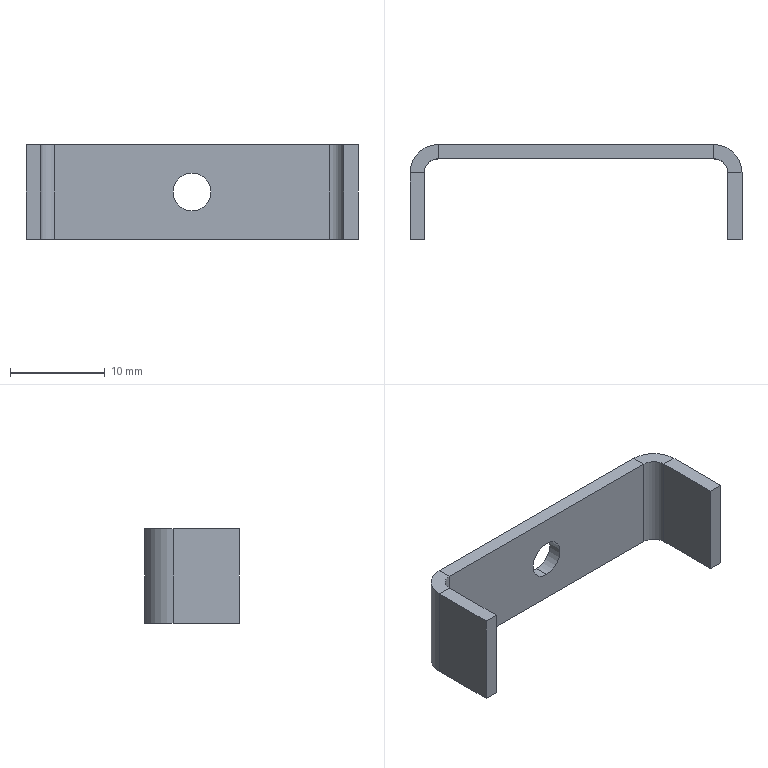Part | SolidWorks | features FlatPattern 1, ICE 1, SMBaseFlange 1, SheetMetal 1 | 1 solid | 24 faces | box 35 x 10 x 10 mm | volume 732.179 mm3 | plane 18 | cylinder 6 | commonest cylinder face diameters 3 x2 4 x2 6 x2
STEP:
#1=CARTESIAN_POINT('',(17.5,8.5,3.));
#2=VERTEX_POINT('',#1);
#3=CARTESIAN_POINT('',(17.5,8.5,7.));
#4=VERTEX_POINT('',#3);
#5=CARTESIAN_POINT('',(17.5,8.5,5.));
#6=DIRECTION('',(0.,1.,0.));
#7=DIRECTION('',(0.,0.,1.));
#8=AXIS2_PLACEMENT_3D('',#5,#6,#7);
#9=CIRCLE('',#8,2.);
#10=EDGE_CURVE('',#2,#4,#9,.T.);
#11=ORIENTED_EDGE('',*,*,#10,.F.);
#12=CARTESIAN_POINT('',(17.5,10.,3.));
#13=VERTEX_POINT('',#12);
#14=CARTESIAN_POINT('',(17.5,0.,3.));
#15=DIRECTION('',(0.,1.,0.));
#16=VECTOR('',#15,1000.);
#17=LINE('',#14,#16);
#18=EDGE_CURVE('',#2,#13,#17,.T.);
#19=ORIENTED_EDGE('',*,*,#18,.T.);
#20=CARTESIAN_POINT('',(17.5,10.,7.));
#21=VERTEX_POINT('',#20);
#22=CARTESIAN_POINT('',(17.5,10.,5.));
#23=DIRECTION('',(0.,1.,0.));
#24=DIRECTION('',(0.,0.,1.));
#25=AXIS2_PLACEMENT_3D('',#22,#23,#24);
#26=CIRCLE('',#25,2.);
#27=EDGE_CURVE('',#13,#21,#26,.T.);
#28=ORIENTED_EDGE('',*,*,#27,.T.);
#29=CARTESIAN_POINT('',(17.5,0.,7.));
#30=DIRECTION('',(0.,1.,0.));
#31=VECTOR('',#30,1000.);
#32=LINE('',#29,#31);
#33=EDGE_CURVE('',#4,#21,#32,.T.);
#34=ORIENTED_EDGE('',*,*,#33,.F.);
#35=EDGE_LOOP('',(#11,#19,#28,#34));
#36=FACE_OUTER_BOUND('',#35,.T.);
#37=CARTESIAN_POINT('',(17.5,0.,5.));
#38=DIRECTION('',(0.,1.,0.));
#39=DIRECTION('',(0.,0.,1.));
#40=AXIS2_PLACEMENT_3D('',#37,#38,#39);
#41=CYLINDRICAL_SURFACE('',#40,2.);
#42=ADVANCED_FACE('',(#36),#41,.F.);
#43=CARTESIAN_POINT('',(3.,10.,10.));
#44=VERTEX_POINT('',#43);
#45=CARTESIAN_POINT('',(3.,8.5,10.));
#46=VERTEX_POINT('',#45);
#47=CARTESIAN_POINT('',(3.,10.,10.));
#48=DIRECTION('',(0.,-1.,0.));
#49=VECTOR('',#48,1000.);
#50=LINE('',#47,#49);
#51=EDGE_CURVE('',#44,#46,#50,.T.);
#52=ORIENTED_EDGE('',*,*,#51,.F.);
#53=CARTESIAN_POINT('',(0.,7.,10.));
#54=VERTEX_POINT('',#53);
#55=CARTESIAN_POINT('',(3.,7.,10.));
#56=DIRECTION('',(0.,0.,-1.));
#57=DIRECTION('',(1.,0.,0.));
#58=AXIS2_PLACEMENT_3D('',#55,#56,#57);
#59=CIRCLE('',#58,3.);
#60=EDGE_CURVE('',#54,#44,#59,.T.);
#61=ORIENTED_EDGE('',*,*,#60,.F.);
#62=CARTESIAN_POINT('',(1.5,7.,10.));
#63=VERTEX_POINT('',#62);
#64=CARTESIAN_POINT('',(1.5,7.,10.));
#65=DIRECTION('',(-1.,0.,0.));
#66=VECTOR('',#65,1000.);
#67=LINE('',#64,#66);
#68=EDGE_CURVE('',#63,#54,#67,.T.);
#69=ORIENTED_EDGE('',*,*,#68,.F.);
#70=CARTESIAN_POINT('',(3.,7.,10.));
#71=DIRECTION('',(0.,0.,-1.));
#72=DIRECTION('',(1.,0.,0.));
#73=AXIS2_PLACEMENT_3D('',#70,#71,#72);
#74=CIRCLE('',#73,1.5);
#75=EDGE_CURVE('',#63,#46,#74,.T.);
#76=ORIENTED_EDGE('',*,*,#75,.T.);
#77=EDGE_LOOP('',(#52,#61,#69,#76));
#78=FACE_OUTER_BOUND('',#77,.T.);
#79=CARTESIAN_POINT('',(3.,10.,10.));
#80=DIRECTION('',(0.,0.,1.));
#81=DIRECTION('',(1.,0.,0.));
#82=AXIS2_PLACEMENT_3D('',#79,#80,#81);
#83=PLANE('',#82);
#84=ADVANCED_FACE('',(#78),#83,.T.);
#85=CARTESIAN_POINT('',(32.,10.,10.));
#86=VERTEX_POINT('',#85);
#87=CARTESIAN_POINT('',(0.,10.,10.));
#88=DIRECTION('',(1.,0.,0.));
#89=VECTOR('',#88,1000.);
#90=LINE('',#87,#89);
#91=EDGE_CURVE('',#44,#86,#90,.T.);
#92=ORIENTED_EDGE('',*,*,#91,.F.);
#93=ORIENTED_EDGE('',*,*,#51,.T.);
#94=CARTESIAN_POINT('',(32.,8.5,10.));
#95=VERTEX_POINT('',#94);
#96=CARTESIAN_POINT('',(0.,8.5,10.));
#97=DIRECTION('',(1.,0.,0.));
#98=VECTOR('',#97,1000.);
#99=LINE('',#96,#98);
#100=EDGE_CURVE('',#46,#95,#99,.T.);
#101=ORIENTED_EDGE('',*,*,#100,.T.);
#102=CARTESIAN_POINT('',(32.,8.5,10.));
#103=DIRECTION('',(0.,1.,0.));
#104=VECTOR('',#103,1000.);
#105=LINE('',#102,#104);
#106=EDGE_CURVE('',#95,#86,#105,.T.);
#107=ORIENTED_EDGE('',*,*,#106,.T.);
#108=EDGE_LOOP('',(#92,#93,#101,#107));
#109=FACE_OUTER_BOUND('',#108,.T.);
#110=CARTESIAN_POINT('',(1.5,7.,10.));
#111=DIRECTION('',(0.,0.,1.));
#112=DIRECTION('',(1.,0.,0.));
#113=AXIS2_PLACEMENT_3D('',#110,#111,#112);
#114=PLANE('',#113);
#115=ADVANCED_FACE('',(#109),#114,.T.);
#116=CARTESIAN_POINT('',(0.,7.,0.));
#117=VERTEX_POINT('',#116);
#118=CARTESIAN_POINT('',(1.5,7.,0.));
#119=VERTEX_POINT('',#118);
#120=CARTESIAN_POINT('',(0.,7.,0.));
#121=DIRECTION('',(1.,0.,0.));
#122=VECTOR('',#121,1000.);
#123=LINE('',#120,#122);
#124=EDGE_CURVE('',#117,#119,#123,.T.);
#125=ORIENTED_EDGE('',*,*,#124,.F.);
#126=CARTESIAN_POINT('',(3.,10.,0.));
#127=VERTEX_POINT('',#126);
#128=CARTESIAN_POINT('',(3.,7.,0.));
#129=DIRECTION('',(0.,0.,-1.));
#130=DIRECTION('',(1.,0.,0.));
#131=AXIS2_PLACEMENT_3D('',#128,#129,#130);
#132=CIRCLE('',#131,3.);
#133=EDGE_CURVE('',#117,#127,#132,.T.);
#134=ORIENTED_EDGE('',*,*,#133,.T.);
#135=CARTESIAN_POINT('',(3.,8.5,0.));
#136=VERTEX_POINT('',#135);
#137=CARTESIAN_POINT('',(3.,8.5,0.));
#138=DIRECTION('',(0.,1.,0.));
#139=VECTOR('',#138,1000.);
#140=LINE('',#137,#139);
#141=EDGE_CURVE('',#136,#127,#140,.T.);
#142=ORIENTED_EDGE('',*,*,#141,.F.);
#143=CARTESIAN_POINT('',(3.,7.,0.));
#144=DIRECTION('',(0.,0.,-1.));
#145=DIRECTION('',(1.,0.,0.));
#146=AXIS2_PLACEMENT_3D('',#143,#144,#145);
#147=CIRCLE('',#146,1.5);
#148=EDGE_CURVE('',#119,#136,#147,.T.);
#149=ORIENTED_EDGE('',*,*,#148,.F.);
#150=EDGE_LOOP('',(#125,#134,#142,#149));
#151=FACE_OUTER_BOUND('',#150,.T.);
#152=CARTESIAN_POINT('',(0.,7.,0.));
#153=DIRECTION('',(0.,0.,-1.));
#154=DIRECTION('',(-1.,0.,0.));
#155=AXIS2_PLACEMENT_3D('',#152,#153,#154);
#156=PLANE('',#155);
#157=ADVANCED_FACE('',(#151),#156,.T.);
#158=CARTESIAN_POINT('',(0.,0.,0.));
#159=VERTEX_POINT('',#158);
#160=CARTESIAN_POINT('',(0.,0.,0.));
#161=DIRECTION('',(0.,1.,0.));
#162=VECTOR('',#161,1000.);
#163=LINE('',#160,#162);
#164=EDGE_CURVE('',#159,#117,#163,.T.);
#165=ORIENTED_EDGE('',*,*,#164,.T.);
#166=ORIENTED_EDGE('',*,*,#124,.T.);
#167=CARTESIAN_POINT('',(1.5,0.,0.));
#168=VERTEX_POINT('',#167);
#169=CARTESIAN_POINT('',(1.5,0.,0.));
#170=DIRECTION('',(0.,1.,0.));
#171=VECTOR('',#170,1000.);
#172=LINE('',#169,#171);
#173=EDGE_CURVE('',#168,#119,#172,.T.);
#174=ORIENTED_EDGE('',*,*,#173,.F.);
#175=CARTESIAN_POINT('',(1.5,0.,0.));
#176=DIRECTION('',(-1.,0.,0.));
#177=VECTOR('',#176,1000.);
#178=LINE('',#175,#177);
#179=EDGE_CURVE('',#168,#159,#178,.T.);
#180=ORIENTED_EDGE('',*,*,#179,.T.);
#181=EDGE_LOOP('',(#165,#166,#174,#180));
#182=FACE_OUTER_BOUND('',#181,.T.);
#183=CARTESIAN_POINT('',(3.,8.5,0.));
#184=DIRECTION('',(0.,0.,-1.));
#185=DIRECTION('',(-1.,0.,0.));
#186=AXIS2_PLACEMENT_3D('',#183,#184,#185);
#187=PLANE('',#186);
#188=ADVANCED_FACE('',(#182),#187,.T.);
#189=CARTESIAN_POINT('',(35.,7.,10.));
#190=VERTEX_POINT('',#189);
#191=CARTESIAN_POINT('',(33.5,7.,10.));
#192=VERTEX_POINT('',#191);
#193=CARTESIAN_POINT('',(35.,7.,10.));
#194=DIRECTION('',(-1.,0.,0.));
#195=VECTOR('',#194,1000.);
#196=LINE('',#193,#195);
#197=EDGE_CURVE('',#190,#192,#196,.T.);
#198=ORIENTED_EDGE('',*,*,#197,.F.);
#199=CARTESIAN_POINT('',(32.,7.,10.));
#200=DIRECTION('',(0.,0.,-1.));
#201=DIRECTION('',(1.,0.,0.));
#202=AXIS2_PLACEMENT_3D('',#199,#200,#201);
#203=CIRCLE('',#202,3.);
#204=EDGE_CURVE('',#86,#190,#203,.T.);
#205=ORIENTED_EDGE('',*,*,#204,.F.);
#206=ORIENTED_EDGE('',*,*,#106,.F.);
#207=CARTESIAN_POINT('',(32.,7.,10.));
#208=DIRECTION('',(0.,0.,-1.));
#209=DIRECTION('',(1.,0.,0.));
#210=AXIS2_PLACEMENT_3D('',#207,#208,#209);
#211=CIRCLE('',#210,1.5);
#212=EDGE_CURVE('',#95,#192,#211,.T.);
#213=ORIENTED_EDGE('',*,*,#212,.T.);
#214=EDGE_LOOP('',(#198,#205,#206,#213));
#215=FACE_OUTER_BOUND('',#214,.T.);
#216=CARTESIAN_POINT('',(35.,7.,10.));
#217=DIRECTION('',(0.,0.,1.));
#218=DIRECTION('',(1.,0.,0.));
#219=AXIS2_PLACEMENT_3D('',#216,#217,#218);
#220=PLANE('',#219);
#221=ADVANCED_FACE('',(#215),#220,.T.);
#222=CARTESIAN_POINT('',(35.,0.,10.));
#223=VERTEX_POINT('',#222);
#224=CARTESIAN_POINT('',(35.,10.,10.));
#225=DIRECTION('',(0.,-1.,0.));
#226=VECTOR('',#225,1000.);
#227=LINE('',#224,#226);
#228=EDGE_CURVE('',#190,#223,#227,.T.);
#229=ORIENTED_EDGE('',*,*,#228,.F.);
#230=ORIENTED_EDGE('',*,*,#197,.T.);
#231=CARTESIAN_POINT('',(33.5,0.,10.));
#232=VERTEX_POINT('',#231);
#233=CARTESIAN_POINT('',(33.5,10.,10.));
#234=DIRECTION('',(0.,-1.,0.));
#235=VECTOR('',#234,1000.);
#236=LINE('',#233,#235);
#237=EDGE_CURVE('',#192,#232,#236,.T.);
#238=ORIENTED_EDGE('',*,*,#237,.T.);
#239=CARTESIAN_POINT('',(35.,0.,10.));
#240=DIRECTION('',(-1.,0.,0.));
#241=VECTOR('',#240,1000.);
#242=LINE('',#239,#241);
#243=EDGE_CURVE('',#223,#232,#242,.T.);
#244=ORIENTED_EDGE('',*,*,#243,.F.);
#245=EDGE_LOOP('',(#229,#230,#238,#244));
#246=FACE_OUTER_BOUND('',#245,.T.);
#247=CARTESIAN_POINT('',(32.,8.5,10.));
#248=DIRECTION('',(0.,0.,1.));
#249=DIRECTION('',(1.,0.,0.));
#250=AXIS2_PLACEMENT_3D('',#247,#248,#249);
#251=PLANE('',#250);
#252=ADVANCED_FACE('',(#246),#251,.T.);
#253=CARTESIAN_POINT('',(32.,10.,0.));
#254=VERTEX_POINT('',#253);
#255=CARTESIAN_POINT('',(32.,8.5,0.));
#256=VERTEX_POINT('',#255);
#257=CARTESIAN_POINT('',(32.,10.,0.));
#258=DIRECTION('',(0.,-1.,0.));
#259=VECTOR('',#258,1000.);
#260=LINE('',#257,#259);
#261=EDGE_CURVE('',#254,#256,#260,.T.);
#262=ORIENTED_EDGE('',*,*,#261,.F.);
#263=CARTESIAN_POINT('',(35.,7.,0.));
#264=VERTEX_POINT('',#263);
#265=CARTESIAN_POINT('',(32.,7.,0.));
#266=DIRECTION('',(0.,0.,-1.));
#267=DIRECTION('',(1.,0.,0.));
#268=AXIS2_PLACEMENT_3D('',#265,#266,#267);
#269=CIRCLE('',#268,3.);
#270=EDGE_CURVE('',#254,#264,#269,.T.);
#271=ORIENTED_EDGE('',*,*,#270,.T.);
#272=CARTESIAN_POINT('',(33.5,7.,0.));
#273=VERTEX_POINT('',#272);
#274=CARTESIAN_POINT('',(33.5,7.,0.));
#275=DIRECTION('',(1.,0.,0.));
#276=VECTOR('',#275,1000.);
#277=LINE('',#274,#276);
#278=EDGE_CURVE('',#273,#264,#277,.T.);
#279=ORIENTED_EDGE('',*,*,#278,.F.);
#280=CARTESIAN_POINT('',(32.,7.,0.));
#281=DIRECTION('',(0.,0.,-1.));
#282=DIRECTION('',(1.,0.,0.));
#283=AXIS2_PLACEMENT_3D('',#280,#281,#282);
#284=CIRCLE('',#283,1.5);
#285=EDGE_CURVE('',#256,#273,#284,.T.);
#286=ORIENTED_EDGE('',*,*,#285,.F.);
#287=EDGE_LOOP('',(#262,#271,#279,#286));
#288=FACE_OUTER_BOUND('',#287,.T.);
#289=CARTESIAN_POINT('',(32.,10.,0.));
#290=DIRECTION('',(0.,0.,-1.));
#291=DIRECTION('',(-1.,0.,0.));
#292=AXIS2_PLACEMENT_3D('',#289,#290,#291);
#293=PLANE('',#292);
#294=ADVANCED_FACE('',(#288),#293,.T.);
#295=CARTESIAN_POINT('',(0.,10.,0.));
#296=DIRECTION('',(1.,0.,0.));
#297=VECTOR('',#296,1000.);
#298=LINE('',#295,#297);
#299=EDGE_CURVE('',#127,#254,#298,.T.);
#300=ORIENTED_EDGE('',*,*,#299,.T.);
#301=ORIENTED_EDGE('',*,*,#261,.T.);
#302=CARTESIAN_POINT('',(0.,8.5,0.));
#303=DIRECTION('',(1.,0.,0.));
#304=VECTOR('',#303,1000.);
#305=LINE('',#302,#304);
#306=EDGE_CURVE('',#136,#256,#305,.T.);
#307=ORIENTED_EDGE('',*,*,#306,.F.);
#308=ORIENTED_EDGE('',*,*,#141,.T.);
#309=EDGE_LOOP('',(#300,#301,#307,#308));
#310=FACE_OUTER_BOUND('',#309,.T.);
#311=CARTESIAN_POINT('',(33.5,7.,0.));
#312=DIRECTION('',(0.,0.,-1.));
#313=DIRECTION('',(-1.,0.,0.));
#314=AXIS2_PLACEMENT_3D('',#311,#312,#313);
#315=PLANE('',#314);
#316=ADVANCED_FACE('',(#310),#315,.T.);
#317=CARTESIAN_POINT('',(33.5,0.,0.));
#318=VERTEX_POINT('',#317);
#319=CARTESIAN_POINT('',(33.5,10.,0.));
#320=DIRECTION('',(0.,-1.,0.));
#321=VECTOR('',#320,1000.);
#322=LINE('',#319,#321);
#323=EDGE_CURVE('',#273,#318,#322,.T.);
#324=ORIENTED_EDGE('',*,*,#323,.T.);
#325=CARTESIAN_POINT('',(33.5,0.,10.));
#326=DIRECTION('',(0.,0.,-1.));
#327=VECTOR('',#326,1000.);
#328=LINE('',#325,#327);
#329=EDGE_CURVE('',#232,#318,#328,.T.);
#330=ORIENTED_EDGE('',*,*,#329,.F.);
#331=ORIENTED_EDGE('',*,*,#237,.F.);
#332=CARTESIAN_POINT('',(33.5,7.,10.));
#333=DIRECTION('',(0.,0.,-1.));
#334=VECTOR('',#333,1000.);
#335=LINE('',#332,#334);
#336=EDGE_CURVE('',#192,#273,#335,.T.);
#337=ORIENTED_EDGE('',*,*,#336,.T.);
#338=EDGE_LOOP('',(#324,#330,#331,#337));
#339=FACE_OUTER_BOUND('',#338,.T.);
#340=CARTESIAN_POINT('',(33.5,10.,10.));
#341=DIRECTION('',(1.,0.,0.));
#342=DIRECTION('',(0.,0.,-1.));
#343=AXIS2_PLACEMENT_3D('',#340,#341,#342);
#344=PLANE('',#343);
#345=ADVANCED_FACE('',(#339),#344,.F.);
#346=CARTESIAN_POINT('',(35.,0.,0.));
#347=VERTEX_POINT('',#346);
#348=CARTESIAN_POINT('',(35.,0.,0.));
#349=DIRECTION('',(-1.,0.,0.));
#350=VECTOR('',#349,1000.);
#351=LINE('',#348,#350);
#352=EDGE_CURVE('',#347,#318,#351,.T.);
#353=ORIENTED_EDGE('',*,*,#352,.F.);
#354=CARTESIAN_POINT('',(35.,0.,10.));
#355=DIRECTION('',(0.,0.,-1.));
#356=VECTOR('',#355,1000.);
#357=LINE('',#354,#356);
#358=EDGE_CURVE('',#223,#347,#357,.T.);
#359=ORIENTED_EDGE('',*,*,#358,.F.);
#360=ORIENTED_EDGE('',*,*,#243,.T.);
#361=ORIENTED_EDGE('',*,*,#329,.T.);
#362=EDGE_LOOP('',(#353,#359,#360,#361));
#363=FACE_OUTER_BOUND('',#362,.T.);
#364=CARTESIAN_POINT('',(35.,0.,10.));
#365=DIRECTION('',(0.,-1.,0.));
#366=DIRECTION('',(1.,0.,0.));
#367=AXIS2_PLACEMENT_3D('',#364,#365,#366);
#368=PLANE('',#367);
#369=ADVANCED_FACE('',(#363),#368,.T.);
#370=CARTESIAN_POINT('',(35.,10.,0.));
#371=DIRECTION('',(0.,-1.,0.));
#372=VECTOR('',#371,1000.);
#373=LINE('',#370,#372);
#374=EDGE_CURVE('',#264,#347,#373,.T.);
#375=ORIENTED_EDGE('',*,*,#374,.F.);
#376=CARTESIAN_POINT('',(35.,7.,10.));
#377=DIRECTION('',(0.,0.,-1.));
#378=VECTOR('',#377,1000.);
#379=LINE('',#376,#378);
#380=EDGE_CURVE('',#190,#264,#379,.T.);
#381=ORIENTED_EDGE('',*,*,#380,.F.);
#382=ORIENTED_EDGE('',*,*,#228,.T.);
#383=ORIENTED_EDGE('',*,*,#358,.T.);
#384=EDGE_LOOP('',(#375,#381,#382,#383));
#385=FACE_OUTER_BOUND('',#384,.T.);
#386=CARTESIAN_POINT('',(35.,10.,10.));
#387=DIRECTION('',(1.,0.,0.));
#388=DIRECTION('',(0.,0.,-1.));
#389=AXIS2_PLACEMENT_3D('',#386,#387,#388);
#390=PLANE('',#389);
#391=ADVANCED_FACE('',(#385),#390,.T.);
#392=ORIENTED_EDGE('',*,*,#270,.F.);
#393=CARTESIAN_POINT('',(32.,10.,10.));
#394=DIRECTION('',(0.,0.,-1.));
#395=VECTOR('',#394,1000.);
#396=LINE('',#393,#395);
#397=EDGE_CURVE('',#86,#254,#396,.T.);
#398=ORIENTED_EDGE('',*,*,#397,.F.);
#399=ORIENTED_EDGE('',*,*,#204,.T.);
#400=ORIENTED_EDGE('',*,*,#380,.T.);
#401=EDGE_LOOP('',(#392,#398,#399,#400));
#402=FACE_OUTER_BOUND('',#401,.T.);
#403=CARTESIAN_POINT('',(32.,7.,10.));
#404=DIRECTION('',(0.,0.,-1.));
#405=DIRECTION('',(-1.,0.,0.));
#406=AXIS2_PLACEMENT_3D('',#403,#404,#405);
#407=CYLINDRICAL_SURFACE('',#406,3.);
#408=ADVANCED_FACE('',(#402),#407,.T.);
#409=CARTESIAN_POINT('',(17.5,10.,5.));
#410=DIRECTION('',(0.,1.,0.));
#411=DIRECTION('',(0.,0.,1.));
#412=AXIS2_PLACEMENT_3D('',#409,#410,#411);
#413=CIRCLE('',#412,2.);
#414=EDGE_CURVE('',#21,#13,#413,.T.);
#415=ORIENTED_EDGE('',*,*,#414,.F.);
#416=ORIENTED_EDGE('',*,*,#27,.F.);
#417=EDGE_LOOP('',(#415,#416));
#418=FACE_BOUND('',#417,.T.);
#419=ORIENTED_EDGE('',*,*,#299,.F.);
#420=CARTESIAN_POINT('',(3.,10.,10.));
#421=DIRECTION('',(0.,0.,-1.));
#422=VECTOR('',#421,1000.);
#423=LINE('',#420,#422);
#424=EDGE_CURVE('',#44,#127,#423,.T.);
#425=ORIENTED_EDGE('',*,*,#424,.F.);
#426=ORIENTED_EDGE('',*,*,#91,.T.);
#427=ORIENTED_EDGE('',*,*,#397,.T.);
#428=EDGE_LOOP('',(#419,#425,#426,#427));
#429=FACE_OUTER_BOUND('',#428,.T.);
#430=CARTESIAN_POINT('',(0.,10.,10.));
#431=DIRECTION('',(0.,1.,0.));
#432=DIRECTION('',(0.,0.,1.));
#433=AXIS2_PLACEMENT_3D('',#430,#431,#432);
#434=PLANE('',#433);
#435=ADVANCED_FACE('',(#418,#429),#434,.T.);
#436=ORIENTED_EDGE('',*,*,#133,.F.);
#437=CARTESIAN_POINT('',(0.,7.,10.));
#438=DIRECTION('',(0.,0.,-1.));
#439=VECTOR('',#438,1000.);
#440=LINE('',#437,#439);
#441=EDGE_CURVE('',#54,#117,#440,.T.);
#442=ORIENTED_EDGE('',*,*,#441,.F.);
#443=ORIENTED_EDGE('',*,*,#60,.T.);
#444=ORIENTED_EDGE('',*,*,#424,.T.);
#445=EDGE_LOOP('',(#436,#442,#443,#444));
#446=FACE_OUTER_BOUND('',#445,.T.);
#447=CARTESIAN_POINT('',(3.,7.,10.));
#448=DIRECTION('',(0.,0.,-1.));
#449=DIRECTION('',(-1.,0.,0.));
#450=AXIS2_PLACEMENT_3D('',#447,#448,#449);
#451=CYLINDRICAL_SURFACE('',#450,3.);
#452=ADVANCED_FACE('',(#446),#451,.T.);
#453=ORIENTED_EDGE('',*,*,#164,.F.);
#454=CARTESIAN_POINT('',(0.,0.,10.));
#455=VERTEX_POINT('',#454);
#456=CARTESIAN_POINT('',(0.,0.,10.));
#457=DIRECTION('',(0.,0.,-1.));
#458=VECTOR('',#457,1000.);
#459=LINE('',#456,#458);
#460=EDGE_CURVE('',#455,#159,#459,.T.);
#461=ORIENTED_EDGE('',*,*,#460,.F.);
#462=CARTESIAN_POINT('',(0.,0.,10.));
#463=DIRECTION('',(0.,1.,0.));
#464=VECTOR('',#463,1000.);
#465=LINE('',#462,#464);
#466=EDGE_CURVE('',#455,#54,#465,.T.);
#467=ORIENTED_EDGE('',*,*,#466,.T.);
#468=ORIENTED_EDGE('',*,*,#441,.T.);
#469=EDGE_LOOP('',(#453,#461,#467,#468));
#470=FACE_OUTER_BOUND('',#469,.T.);
#471=CARTESIAN_POINT('',(0.,0.,10.));
#472=DIRECTION('',(-1.,0.,0.));
#473=DIRECTION('',(0.,0.,1.));
#474=AXIS2_PLACEMENT_3D('',#471,#472,#473);
#475=PLANE('',#474);
#476=ADVANCED_FACE('',(#470),#475,.T.);
#477=ORIENTED_EDGE('',*,*,#179,.F.);
#478=CARTESIAN_POINT('',(1.5,0.,10.));
#479=VERTEX_POINT('',#478);
#480=CARTESIAN_POINT('',(1.5,0.,10.));
#481=DIRECTION('',(0.,0.,-1.));
#482=VECTOR('',#481,1000.);
#483=LINE('',#480,#482);
#484=EDGE_CURVE('',#479,#168,#483,.T.);
#485=ORIENTED_EDGE('',*,*,#484,.F.);
#486=CARTESIAN_POINT('',(1.5,0.,10.));
#487=DIRECTION('',(-1.,0.,0.));
#488=VECTOR('',#487,1000.);
#489=LINE('',#486,#488);
#490=EDGE_CURVE('',#479,#455,#489,.T.);
#491=ORIENTED_EDGE('',*,*,#490,.T.);
#492=ORIENTED_EDGE('',*,*,#460,.T.);
#493=EDGE_LOOP('',(#477,#485,#491,#492));
#494=FACE_OUTER_BOUND('',#493,.T.);
#495=CARTESIAN_POINT('',(1.5,0.,10.));
#496=DIRECTION('',(0.,-1.,0.));
#497=DIRECTION('',(0.,0.,-1.));
#498=AXIS2_PLACEMENT_3D('',#495,#496,#497);
#499=PLANE('',#498);
#500=ADVANCED_FACE('',(#494),#499,.T.);
#501=ORIENTED_EDGE('',*,*,#173,.T.);
#502=CARTESIAN_POINT('',(1.5,7.,10.));
#503=DIRECTION('',(0.,0.,-1.));
#504=VECTOR('',#503,1000.);
#505=LINE('',#502,#504);
#506=EDGE_CURVE('',#63,#119,#505,.T.);
#507=ORIENTED_EDGE('',*,*,#506,.F.);
#508=CARTESIAN_POINT('',(1.5,0.,10.));
#509=DIRECTION('',(0.,1.,0.));
#510=VECTOR('',#509,1000.);
#511=LINE('',#508,#510);
#512=EDGE_CURVE('',#479,#63,#511,.T.);
#513=ORIENTED_EDGE('',*,*,#512,.F.);
#514=ORIENTED_EDGE('',*,*,#484,.T.);
#515=EDGE_LOOP('',(#501,#507,#513,#514));
#516=FACE_OUTER_BOUND('',#515,.T.);
#517=CARTESIAN_POINT('',(1.5,0.,10.));
#518=DIRECTION('',(-1.,0.,0.));
#519=DIRECTION('',(0.,0.,1.));
#520=AXIS2_PLACEMENT_3D('',#517,#518,#519);
#521=PLANE('',#520);
#522=ADVANCED_FACE('',(#516),#521,.F.);
#523=ORIENTED_EDGE('',*,*,#148,.T.);
#524=CARTESIAN_POINT('',(3.,8.5,10.));
#525=DIRECTION('',(0.,0.,-1.));
#526=VECTOR('',#525,1000.);
#527=LINE('',#524,#526);
#528=EDGE_CURVE('',#46,#136,#527,.T.);
#529=ORIENTED_EDGE('',*,*,#528,.F.);
#530=ORIENTED_EDGE('',*,*,#75,.F.);
#531=ORIENTED_EDGE('',*,*,#506,.T.);
#532=EDGE_LOOP('',(#523,#529,#530,#531));
#533=FACE_OUTER_BOUND('',#532,.T.);
#534=CARTESIAN_POINT('',(3.,7.,10.));
#535=DIRECTION('',(0.,0.,-1.));
#536=DIRECTION('',(-1.,0.,0.));
#537=AXIS2_PLACEMENT_3D('',#534,#535,#536);
#538=CYLINDRICAL_SURFACE('',#537,1.5);
#539=ADVANCED_FACE('',(#533),#538,.F.);
#540=CARTESIAN_POINT('',(17.5,8.5,5.));
#541=DIRECTION('',(0.,1.,0.));
#542=DIRECTION('',(0.,0.,1.));
#543=AXIS2_PLACEMENT_3D('',#540,#541,#542);
#544=CIRCLE('',#543,2.);
#545=EDGE_CURVE('',#4,#2,#544,.T.);
#546=ORIENTED_EDGE('',*,*,#545,.T.);
#547=ORIENTED_EDGE('',*,*,#10,.T.);
#548=EDGE_LOOP('',(#546,#547));
#549=FACE_BOUND('',#548,.T.);
#550=ORIENTED_EDGE('',*,*,#306,.T.);
#551=CARTESIAN_POINT('',(32.,8.5,10.));
#552=DIRECTION('',(0.,0.,-1.));
#553=VECTOR('',#552,1000.);
#554=LINE('',#551,#553);
#555=EDGE_CURVE('',#95,#256,#554,.T.);
#556=ORIENTED_EDGE('',*,*,#555,.F.);
#557=ORIENTED_EDGE('',*,*,#100,.F.);
#558=ORIENTED_EDGE('',*,*,#528,.T.);
#559=EDGE_LOOP('',(#550,#556,#557,#558));
#560=FACE_OUTER_BOUND('',#559,.T.);
#561=CARTESIAN_POINT('',(0.,8.5,10.));
#562=DIRECTION('',(0.,1.,0.));
#563=DIRECTION('',(0.,0.,1.));
#564=AXIS2_PLACEMENT_3D('',#561,#562,#563);
#565=PLANE('',#564);
#566=ADVANCED_FACE('',(#549,#560),#565,.F.);
#567=ORIENTED_EDGE('',*,*,#285,.T.);
#568=ORIENTED_EDGE('',*,*,#336,.F.);
#569=ORIENTED_EDGE('',*,*,#212,.F.);
#570=ORIENTED_EDGE('',*,*,#555,.T.);
#571=EDGE_LOOP('',(#567,#568,#569,#570));
#572=FACE_OUTER_BOUND('',#571,.T.);
#573=CARTESIAN_POINT('',(32.,7.,10.));
#574=DIRECTION('',(0.,0.,-1.));
#575=DIRECTION('',(-1.,0.,0.));
#576=AXIS2_PLACEMENT_3D('',#573,#574,#575);
#577=CYLINDRICAL_SURFACE('',#576,1.5);
#578=ADVANCED_FACE('',(#572),#577,.F.);
#579=ORIENTED_EDGE('',*,*,#512,.T.);
#580=ORIENTED_EDGE('',*,*,#68,.T.);
#581=ORIENTED_EDGE('',*,*,#466,.F.);
#582=ORIENTED_EDGE('',*,*,#490,.F.);
#583=EDGE_LOOP('',(#579,#580,#581,#582));
#584=FACE_OUTER_BOUND('',#583,.T.);
#585=CARTESIAN_POINT('',(32.,7.,10.));
#586=DIRECTION('',(0.,0.,1.));
#587=DIRECTION('',(1.,0.,0.));
#588=AXIS2_PLACEMENT_3D('',#585,#586,#587);
#589=PLANE('',#588);
#590=ADVANCED_FACE('',(#584),#589,.T.);
#591=ORIENTED_EDGE('',*,*,#323,.F.);
#592=ORIENTED_EDGE('',*,*,#278,.T.);
#593=ORIENTED_EDGE('',*,*,#374,.T.);
#594=ORIENTED_EDGE('',*,*,#352,.T.);
#595=EDGE_LOOP('',(#591,#592,#593,#594));
#596=FACE_OUTER_BOUND('',#595,.T.);
#597=CARTESIAN_POINT('',(32.,7.,0.));
#598=DIRECTION('',(0.,0.,1.));
#599=DIRECTION('',(1.,0.,0.));
#600=AXIS2_PLACEMENT_3D('',#597,#598,#599);
#601=PLANE('',#600);
#602=ADVANCED_FACE('',(#596),#601,.F.);
#603=ORIENTED_EDGE('',*,*,#18,.F.);
#604=ORIENTED_EDGE('',*,*,#545,.F.);
#605=ORIENTED_EDGE('',*,*,#33,.T.);
#606=ORIENTED_EDGE('',*,*,#414,.T.);
#607=EDGE_LOOP('',(#603,#604,#605,#606));
#608=FACE_OUTER_BOUND('',#607,.T.);
#609=CARTESIAN_POINT('',(17.5,0.,5.));
#610=DIRECTION('',(0.,1.,0.));
#611=DIRECTION('',(0.,0.,1.));
#612=AXIS2_PLACEMENT_3D('',#609,#610,#611);
#613=CYLINDRICAL_SURFACE('',#612,2.);
#614=ADVANCED_FACE('',(#608),#613,.F.);
#615=CLOSED_SHELL('',(#42,#84,#115,#157,#188,#221,#252,#294,#316,#345,#369,#391,#408,#435,#452,#476,#500,#522,#539,#566,#578,#590,#602,#614));
#616=MANIFOLD_SOLID_BREP('',#615);
#617=CARTESIAN_POINT('',(0.,0.,0.));
#618=DIRECTION('',(0.,0.,1.));
#619=DIRECTION('',(1.,0.,0.));
#620=AXIS2_PLACEMENT_3D('',#617,#618,#619);
#621=(LENGTH_UNIT()NAMED_UNIT(*)SI_UNIT(.MILLI.,.METRE.));
#622=UNCERTAINTY_MEASURE_WITH_UNIT(LENGTH_MEASURE(0.00001),#621,'','');
#623=(NAMED_UNIT(*)PLANE_ANGLE_UNIT()SI_UNIT($,.RADIAN.));
#624=(NAMED_UNIT(*)SI_UNIT($,.STERADIAN.)SOLID_ANGLE_UNIT());
#625=(GEOMETRIC_REPRESENTATION_CONTEXT(3)GLOBAL_UNCERTAINTY_ASSIGNED_CONTEXT((#622))GLOBAL_UNIT_ASSIGNED_CONTEXT((#621,#623,#624))REPRESENTATION_CONTEXT('',''));
#626=ADVANCED_BREP_SHAPE_REPRESENTATION('',(#616,#620),#625);